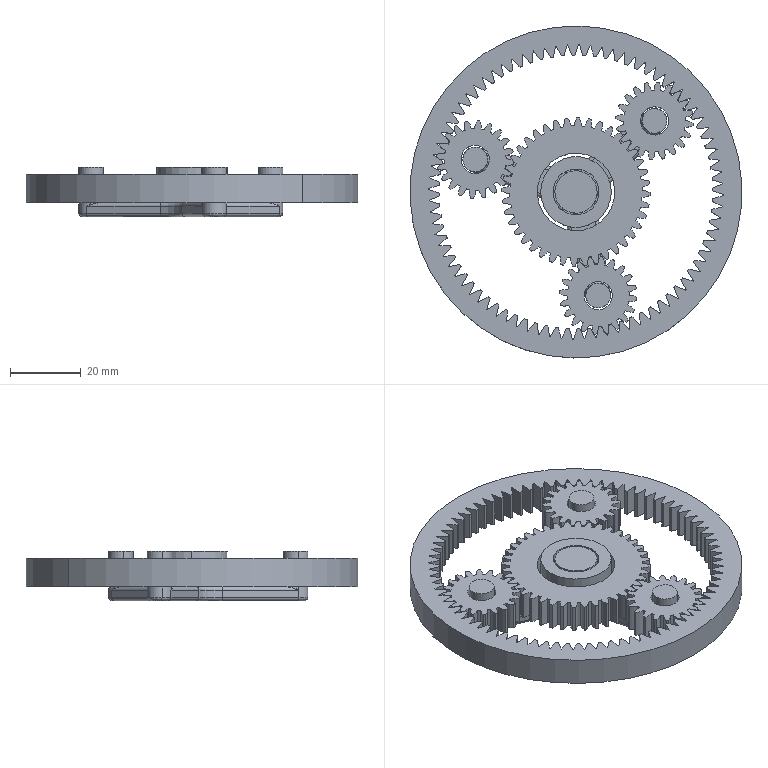Part | SolidWorks | features Attribute 48 | 8 solids | 803 faces | box 94 x 94 x 14 mm | volume 35546 mm3 | cylinder 398 | spline 366 | plane 25 | torus 14 | commonest cylinder face diameters 77.5 x81 83.365 x80 22 x62 17.5 x60 37.5 x40 42 x40